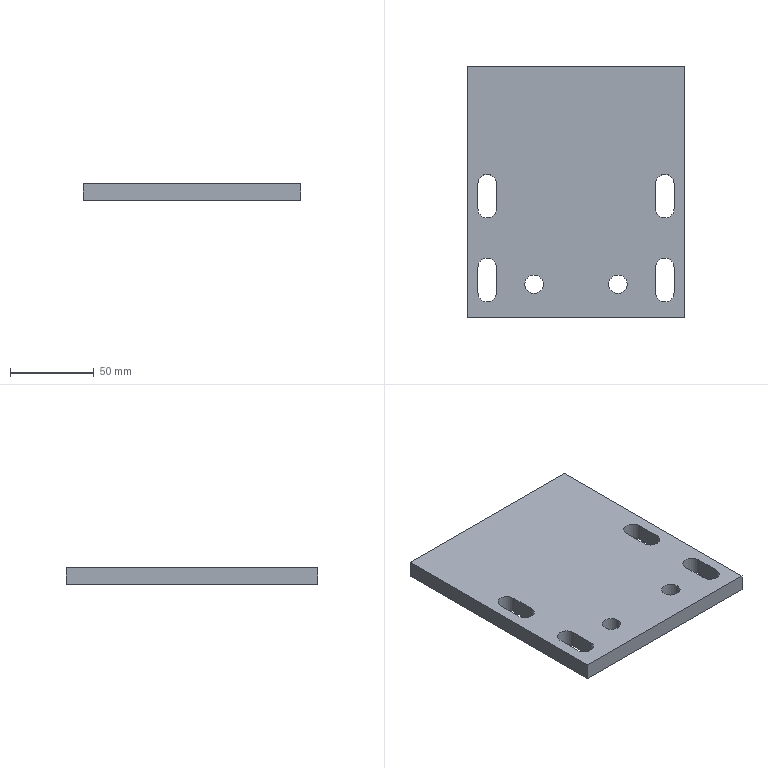Part | SolidWorks | features HoleWzd 2, ICE 2, Extrusion 1 | 1 solid | 26 faces | box 130 x 150 x 10 mm | volume 182698 mm3 | plane 14 | cylinder 12 | commonest cylinder face diameters 11 x12
STEP:
#1=CARTESIAN_POINT('',(34.5,20.,0.));
#2=VERTEX_POINT('',#1);
#3=CARTESIAN_POINT('',(45.5,20.,0.));
#4=VERTEX_POINT('',#3);
#5=CARTESIAN_POINT('',(40.,20.,0.));
#6=DIRECTION('',(0.,0.,1.));
#7=DIRECTION('',(1.,0.,0.));
#8=AXIS2_PLACEMENT_3D('',#5,#6,#7);
#9=CIRCLE('',#8,5.5);
#10=EDGE_CURVE('',#2,#4,#9,.T.);
#11=ORIENTED_EDGE('',*,*,#10,.F.);
#12=CARTESIAN_POINT('',(34.5,20.,10.));
#13=VERTEX_POINT('',#12);
#14=CARTESIAN_POINT('',(34.5,20.,10.));
#15=DIRECTION('',(0.,0.,1.));
#16=VECTOR('',#15,1000.);
#17=LINE('',#14,#16);
#18=EDGE_CURVE('',#2,#13,#17,.T.);
#19=ORIENTED_EDGE('',*,*,#18,.T.);
#20=CARTESIAN_POINT('',(45.5,20.,10.));
#21=VERTEX_POINT('',#20);
#22=CARTESIAN_POINT('',(40.,20.,10.));
#23=DIRECTION('',(0.,0.,1.));
#24=DIRECTION('',(1.,0.,0.));
#25=AXIS2_PLACEMENT_3D('',#22,#23,#24);
#26=CIRCLE('',#25,5.5);
#27=EDGE_CURVE('',#13,#21,#26,.T.);
#28=ORIENTED_EDGE('',*,*,#27,.T.);
#29=CARTESIAN_POINT('',(45.5,20.,10.));
#30=DIRECTION('',(0.,0.,1.));
#31=VECTOR('',#30,1000.);
#32=LINE('',#29,#31);
#33=EDGE_CURVE('',#4,#21,#32,.T.);
#34=ORIENTED_EDGE('',*,*,#33,.F.);
#35=EDGE_LOOP('',(#11,#19,#28,#34));
#36=FACE_OUTER_BOUND('',#35,.T.);
#37=CARTESIAN_POINT('',(40.,20.,10.));
#38=DIRECTION('',(0.,0.,1.));
#39=DIRECTION('',(1.,0.,0.));
#40=AXIS2_PLACEMENT_3D('',#37,#38,#39);
#41=CYLINDRICAL_SURFACE('',#40,5.5);
#42=ADVANCED_FACE('',(#36),#41,.F.);
#43=CARTESIAN_POINT('',(84.5,20.,0.));
#44=VERTEX_POINT('',#43);
#45=CARTESIAN_POINT('',(95.5,20.,0.));
#46=VERTEX_POINT('',#45);
#47=CARTESIAN_POINT('',(90.,20.,0.));
#48=DIRECTION('',(0.,0.,1.));
#49=DIRECTION('',(1.,0.,0.));
#50=AXIS2_PLACEMENT_3D('',#47,#48,#49);
#51=CIRCLE('',#50,5.5);
#52=EDGE_CURVE('',#44,#46,#51,.T.);
#53=ORIENTED_EDGE('',*,*,#52,.F.);
#54=CARTESIAN_POINT('',(84.5,20.,10.));
#55=VERTEX_POINT('',#54);
#56=CARTESIAN_POINT('',(84.5,20.,10.));
#57=DIRECTION('',(0.,0.,1.));
#58=VECTOR('',#57,1000.);
#59=LINE('',#56,#58);
#60=EDGE_CURVE('',#44,#55,#59,.T.);
#61=ORIENTED_EDGE('',*,*,#60,.T.);
#62=CARTESIAN_POINT('',(95.5,20.,10.));
#63=VERTEX_POINT('',#62);
#64=CARTESIAN_POINT('',(90.,20.,10.));
#65=DIRECTION('',(0.,0.,1.));
#66=DIRECTION('',(1.,0.,0.));
#67=AXIS2_PLACEMENT_3D('',#64,#65,#66);
#68=CIRCLE('',#67,5.5);
#69=EDGE_CURVE('',#55,#63,#68,.T.);
#70=ORIENTED_EDGE('',*,*,#69,.T.);
#71=CARTESIAN_POINT('',(95.5,20.,10.));
#72=DIRECTION('',(0.,0.,1.));
#73=VECTOR('',#72,1000.);
#74=LINE('',#71,#73);
#75=EDGE_CURVE('',#46,#63,#74,.T.);
#76=ORIENTED_EDGE('',*,*,#75,.F.);
#77=EDGE_LOOP('',(#53,#61,#70,#76));
#78=FACE_OUTER_BOUND('',#77,.T.);
#79=CARTESIAN_POINT('',(90.,20.,10.));
#80=DIRECTION('',(0.,0.,1.));
#81=DIRECTION('',(1.,0.,0.));
#82=AXIS2_PLACEMENT_3D('',#79,#80,#81);
#83=CYLINDRICAL_SURFACE('',#82,5.5);
#84=ADVANCED_FACE('',(#78),#83,.F.);
#85=CARTESIAN_POINT('',(0.,150.,0.));
#86=VERTEX_POINT('',#85);
#87=CARTESIAN_POINT('',(0.,0.,0.));
#88=VERTEX_POINT('',#87);
#89=CARTESIAN_POINT('',(0.,0.,0.));
#90=DIRECTION('',(0.,-1.,0.));
#91=VECTOR('',#90,1000.);
#92=LINE('',#89,#91);
#93=EDGE_CURVE('',#86,#88,#92,.T.);
#94=ORIENTED_EDGE('',*,*,#93,.T.);
#95=CARTESIAN_POINT('',(0.,0.,10.));
#96=VERTEX_POINT('',#95);
#97=CARTESIAN_POINT('',(0.,0.,10.));
#98=DIRECTION('',(0.,0.,-1.));
#99=VECTOR('',#98,1000.);
#100=LINE('',#97,#99);
#101=EDGE_CURVE('',#96,#88,#100,.T.);
#102=ORIENTED_EDGE('',*,*,#101,.F.);
#103=CARTESIAN_POINT('',(0.,150.,10.));
#104=VERTEX_POINT('',#103);
#105=CARTESIAN_POINT('',(0.,0.,10.));
#106=DIRECTION('',(0.,-1.,0.));
#107=VECTOR('',#106,1000.);
#108=LINE('',#105,#107);
#109=EDGE_CURVE('',#104,#96,#108,.T.);
#110=ORIENTED_EDGE('',*,*,#109,.F.);
#111=CARTESIAN_POINT('',(0.,150.,0.));
#112=DIRECTION('',(0.,0.,1.));
#113=VECTOR('',#112,1000.);
#114=LINE('',#111,#113);
#115=EDGE_CURVE('',#86,#104,#114,.T.);
#116=ORIENTED_EDGE('',*,*,#115,.F.);
#117=EDGE_LOOP('',(#94,#102,#110,#116));
#118=FACE_OUTER_BOUND('',#117,.T.);
#119=CARTESIAN_POINT('',(0.,0.,10.));
#120=DIRECTION('',(1.,0.,0.));
#121=DIRECTION('',(0.,0.,-1.));
#122=AXIS2_PLACEMENT_3D('',#119,#120,#121);
#123=PLANE('',#122);
#124=ADVANCED_FACE('',(#118),#123,.F.);
#125=CARTESIAN_POINT('',(130.,0.,0.));
#126=VERTEX_POINT('',#125);
#127=CARTESIAN_POINT('',(0.,0.,0.));
#128=DIRECTION('',(1.,0.,0.));
#129=VECTOR('',#128,1000.);
#130=LINE('',#127,#129);
#131=EDGE_CURVE('',#88,#126,#130,.T.);
#132=ORIENTED_EDGE('',*,*,#131,.T.);
#133=CARTESIAN_POINT('',(130.,0.,10.));
#134=VERTEX_POINT('',#133);
#135=CARTESIAN_POINT('',(130.,0.,10.));
#136=DIRECTION('',(0.,0.,-1.));
#137=VECTOR('',#136,1000.);
#138=LINE('',#135,#137);
#139=EDGE_CURVE('',#134,#126,#138,.T.);
#140=ORIENTED_EDGE('',*,*,#139,.F.);
#141=CARTESIAN_POINT('',(0.,0.,10.));
#142=DIRECTION('',(1.,0.,0.));
#143=VECTOR('',#142,1000.);
#144=LINE('',#141,#143);
#145=EDGE_CURVE('',#96,#134,#144,.T.);
#146=ORIENTED_EDGE('',*,*,#145,.F.);
#147=ORIENTED_EDGE('',*,*,#101,.T.);
#148=EDGE_LOOP('',(#132,#140,#146,#147));
#149=FACE_OUTER_BOUND('',#148,.T.);
#150=CARTESIAN_POINT('',(0.,0.,10.));
#151=DIRECTION('',(0.,1.,0.));
#152=DIRECTION('',(0.,0.,1.));
#153=AXIS2_PLACEMENT_3D('',#150,#151,#152);
#154=PLANE('',#153);
#155=ADVANCED_FACE('',(#149),#154,.F.);
#156=CARTESIAN_POINT('',(130.,150.,0.));
#157=VERTEX_POINT('',#156);
#158=CARTESIAN_POINT('',(130.,0.,0.));
#159=DIRECTION('',(0.,1.,0.));
#160=VECTOR('',#159,1000.);
#161=LINE('',#158,#160);
#162=EDGE_CURVE('',#126,#157,#161,.T.);
#163=ORIENTED_EDGE('',*,*,#162,.T.);
#164=CARTESIAN_POINT('',(130.,150.,10.));
#165=VERTEX_POINT('',#164);
#166=CARTESIAN_POINT('',(130.,150.,10.));
#167=DIRECTION('',(0.,0.,-1.));
#168=VECTOR('',#167,1000.);
#169=LINE('',#166,#168);
#170=EDGE_CURVE('',#165,#157,#169,.T.);
#171=ORIENTED_EDGE('',*,*,#170,.F.);
#172=CARTESIAN_POINT('',(130.,0.,10.));
#173=DIRECTION('',(0.,1.,0.));
#174=VECTOR('',#173,1000.);
#175=LINE('',#172,#174);
#176=EDGE_CURVE('',#134,#165,#175,.T.);
#177=ORIENTED_EDGE('',*,*,#176,.F.);
#178=ORIENTED_EDGE('',*,*,#139,.T.);
#179=EDGE_LOOP('',(#163,#171,#177,#178));
#180=FACE_OUTER_BOUND('',#179,.T.);
#181=CARTESIAN_POINT('',(130.,0.,10.));
#182=DIRECTION('',(-1.,0.,0.));
#183=DIRECTION('',(0.,0.,1.));
#184=AXIS2_PLACEMENT_3D('',#181,#182,#183);
#185=PLANE('',#184);
#186=ADVANCED_FACE('',(#180),#185,.F.);
#187=CARTESIAN_POINT('',(17.5,30.,10.));
#188=VERTEX_POINT('',#187);
#189=CARTESIAN_POINT('',(17.5,15.,10.));
#190=VERTEX_POINT('',#189);
#191=CARTESIAN_POINT('',(17.5,15.,10.));
#192=DIRECTION('',(0.,-1.,0.));
#193=VECTOR('',#192,1000.);
#194=LINE('',#191,#193);
#195=EDGE_CURVE('',#188,#190,#194,.T.);
#196=ORIENTED_EDGE('',*,*,#195,.T.);
#197=CARTESIAN_POINT('',(6.5,15.,10.));
#198=VERTEX_POINT('',#197);
#199=CARTESIAN_POINT('',(12.,15.,10.));
#200=DIRECTION('',(0.,0.,-1.));
#201=DIRECTION('',(-1.,0.,0.));
#202=AXIS2_PLACEMENT_3D('',#199,#200,#201);
#203=CIRCLE('',#202,5.5);
#204=EDGE_CURVE('',#190,#198,#203,.T.);
#205=ORIENTED_EDGE('',*,*,#204,.T.);
#206=CARTESIAN_POINT('',(6.5,30.,10.));
#207=VERTEX_POINT('',#206);
#208=CARTESIAN_POINT('',(6.5,15.,10.));
#209=DIRECTION('',(0.,1.,0.));
#210=VECTOR('',#209,1000.);
#211=LINE('',#208,#210);
#212=EDGE_CURVE('',#198,#207,#211,.T.);
#213=ORIENTED_EDGE('',*,*,#212,.T.);
#214=CARTESIAN_POINT('',(12.,30.,10.));
#215=DIRECTION('',(0.,0.,-1.));
#216=DIRECTION('',(-1.,0.,0.));
#217=AXIS2_PLACEMENT_3D('',#214,#215,#216);
#218=CIRCLE('',#217,5.5);
#219=EDGE_CURVE('',#207,#188,#218,.T.);
#220=ORIENTED_EDGE('',*,*,#219,.T.);
#221=EDGE_LOOP('',(#196,#205,#213,#220));
#222=FACE_BOUND('',#221,.T.);
#223=CARTESIAN_POINT('',(17.5,80.,10.));
#224=VERTEX_POINT('',#223);
#225=CARTESIAN_POINT('',(17.5,65.,10.));
#226=VERTEX_POINT('',#225);
#227=CARTESIAN_POINT('',(17.5,65.,10.));
#228=DIRECTION('',(0.,-1.,0.));
#229=VECTOR('',#228,1000.);
#230=LINE('',#227,#229);
#231=EDGE_CURVE('',#224,#226,#230,.T.);
#232=ORIENTED_EDGE('',*,*,#231,.T.);
#233=CARTESIAN_POINT('',(6.5,65.,10.));
#234=VERTEX_POINT('',#233);
#235=CARTESIAN_POINT('',(12.,65.,10.));
#236=DIRECTION('',(0.,0.,-1.));
#237=DIRECTION('',(-1.,0.,0.));
#238=AXIS2_PLACEMENT_3D('',#235,#236,#237);
#239=CIRCLE('',#238,5.5);
#240=EDGE_CURVE('',#226,#234,#239,.T.);
#241=ORIENTED_EDGE('',*,*,#240,.T.);
#242=CARTESIAN_POINT('',(6.5,80.,10.));
#243=VERTEX_POINT('',#242);
#244=CARTESIAN_POINT('',(6.5,65.,10.));
#245=DIRECTION('',(0.,1.,0.));
#246=VECTOR('',#245,1000.);
#247=LINE('',#244,#246);
#248=EDGE_CURVE('',#234,#243,#247,.T.);
#249=ORIENTED_EDGE('',*,*,#248,.T.);
#250=CARTESIAN_POINT('',(12.,80.,10.));
#251=DIRECTION('',(0.,0.,-1.));
#252=DIRECTION('',(-1.,0.,0.));
#253=AXIS2_PLACEMENT_3D('',#250,#251,#252);
#254=CIRCLE('',#253,5.5);
#255=EDGE_CURVE('',#243,#224,#254,.T.);
#256=ORIENTED_EDGE('',*,*,#255,.T.);
#257=EDGE_LOOP('',(#232,#241,#249,#256));
#258=FACE_BOUND('',#257,.T.);
#259=CARTESIAN_POINT('',(123.5,80.,10.));
#260=VERTEX_POINT('',#259);
#261=CARTESIAN_POINT('',(123.5,65.,10.));
#262=VERTEX_POINT('',#261);
#263=CARTESIAN_POINT('',(123.5,65.,10.));
#264=DIRECTION('',(0.,-1.,0.));
#265=VECTOR('',#264,1000.);
#266=LINE('',#263,#265);
#267=EDGE_CURVE('',#260,#262,#266,.T.);
#268=ORIENTED_EDGE('',*,*,#267,.T.);
#269=CARTESIAN_POINT('',(112.5,65.,10.));
#270=VERTEX_POINT('',#269);
#271=CARTESIAN_POINT('',(118.,65.,10.));
#272=DIRECTION('',(0.,0.,-1.));
#273=DIRECTION('',(-1.,0.,0.));
#274=AXIS2_PLACEMENT_3D('',#271,#272,#273);
#275=CIRCLE('',#274,5.5);
#276=EDGE_CURVE('',#262,#270,#275,.T.);
#277=ORIENTED_EDGE('',*,*,#276,.T.);
#278=CARTESIAN_POINT('',(112.5,80.,10.));
#279=VERTEX_POINT('',#278);
#280=CARTESIAN_POINT('',(112.5,65.,10.));
#281=DIRECTION('',(0.,1.,0.));
#282=VECTOR('',#281,1000.);
#283=LINE('',#280,#282);
#284=EDGE_CURVE('',#270,#279,#283,.T.);
#285=ORIENTED_EDGE('',*,*,#284,.T.);
#286=CARTESIAN_POINT('',(118.,80.,10.));
#287=DIRECTION('',(0.,0.,-1.));
#288=DIRECTION('',(-1.,0.,0.));
#289=AXIS2_PLACEMENT_3D('',#286,#287,#288);
#290=CIRCLE('',#289,5.5);
#291=EDGE_CURVE('',#279,#260,#290,.T.);
#292=ORIENTED_EDGE('',*,*,#291,.T.);
#293=EDGE_LOOP('',(#268,#277,#285,#292));
#294=FACE_BOUND('',#293,.T.);
#295=CARTESIAN_POINT('',(123.5,30.,10.));
#296=VERTEX_POINT('',#295);
#297=CARTESIAN_POINT('',(123.5,15.,10.));
#298=VERTEX_POINT('',#297);
#299=CARTESIAN_POINT('',(123.5,15.,10.));
#300=DIRECTION('',(0.,-1.,0.));
#301=VECTOR('',#300,1000.);
#302=LINE('',#299,#301);
#303=EDGE_CURVE('',#296,#298,#302,.T.);
#304=ORIENTED_EDGE('',*,*,#303,.T.);
#305=CARTESIAN_POINT('',(112.5,15.,10.));
#306=VERTEX_POINT('',#305);
#307=CARTESIAN_POINT('',(118.,15.,10.));
#308=DIRECTION('',(0.,0.,-1.));
#309=DIRECTION('',(-1.,0.,0.));
#310=AXIS2_PLACEMENT_3D('',#307,#308,#309);
#311=CIRCLE('',#310,5.5);
#312=EDGE_CURVE('',#298,#306,#311,.T.);
#313=ORIENTED_EDGE('',*,*,#312,.T.);
#314=CARTESIAN_POINT('',(112.5,30.,10.));
#315=VERTEX_POINT('',#314);
#316=CARTESIAN_POINT('',(112.5,15.,10.));
#317=DIRECTION('',(0.,1.,0.));
#318=VECTOR('',#317,1000.);
#319=LINE('',#316,#318);
#320=EDGE_CURVE('',#306,#315,#319,.T.);
#321=ORIENTED_EDGE('',*,*,#320,.T.);
#322=CARTESIAN_POINT('',(118.,30.,10.));
#323=DIRECTION('',(0.,0.,-1.));
#324=DIRECTION('',(-1.,0.,0.));
#325=AXIS2_PLACEMENT_3D('',#322,#323,#324);
#326=CIRCLE('',#325,5.5);
#327=EDGE_CURVE('',#315,#296,#326,.T.);
#328=ORIENTED_EDGE('',*,*,#327,.T.);
#329=EDGE_LOOP('',(#304,#313,#321,#328));
#330=FACE_BOUND('',#329,.T.);
#331=CARTESIAN_POINT('',(40.,20.,10.));
#332=DIRECTION('',(0.,0.,1.));
#333=DIRECTION('',(1.,0.,0.));
#334=AXIS2_PLACEMENT_3D('',#331,#332,#333);
#335=CIRCLE('',#334,5.5);
#336=EDGE_CURVE('',#21,#13,#335,.T.);
#337=ORIENTED_EDGE('',*,*,#336,.F.);
#338=ORIENTED_EDGE('',*,*,#27,.F.);
#339=EDGE_LOOP('',(#337,#338));
#340=FACE_BOUND('',#339,.T.);
#341=CARTESIAN_POINT('',(90.,20.,10.));
#342=DIRECTION('',(0.,0.,1.));
#343=DIRECTION('',(1.,0.,0.));
#344=AXIS2_PLACEMENT_3D('',#341,#342,#343);
#345=CIRCLE('',#344,5.5);
#346=EDGE_CURVE('',#63,#55,#345,.T.);
#347=ORIENTED_EDGE('',*,*,#346,.F.);
#348=ORIENTED_EDGE('',*,*,#69,.F.);
#349=EDGE_LOOP('',(#347,#348));
#350=FACE_BOUND('',#349,.T.);
#351=ORIENTED_EDGE('',*,*,#109,.T.);
#352=ORIENTED_EDGE('',*,*,#145,.T.);
#353=ORIENTED_EDGE('',*,*,#176,.T.);
#354=CARTESIAN_POINT('',(0.,150.,10.));
#355=DIRECTION('',(1.,0.,0.));
#356=VECTOR('',#355,1000.);
#357=LINE('',#354,#356);
#358=EDGE_CURVE('',#104,#165,#357,.T.);
#359=ORIENTED_EDGE('',*,*,#358,.F.);
#360=EDGE_LOOP('',(#351,#352,#353,#359));
#361=FACE_OUTER_BOUND('',#360,.T.);
#362=CARTESIAN_POINT('',(0.,0.,10.));
#363=DIRECTION('',(0.,0.,-1.));
#364=DIRECTION('',(-1.,0.,0.));
#365=AXIS2_PLACEMENT_3D('',#362,#363,#364);
#366=PLANE('',#365);
#367=ADVANCED_FACE('',(#222,#258,#294,#330,#340,#350,#361),#366,.F.);
#368=CARTESIAN_POINT('',(17.5,15.,0.));
#369=VERTEX_POINT('',#368);
#370=CARTESIAN_POINT('',(6.5,15.,0.));
#371=VERTEX_POINT('',#370);
#372=CARTESIAN_POINT('',(12.,15.,0.));
#373=DIRECTION('',(0.,0.,-1.));
#374=DIRECTION('',(-1.,0.,0.));
#375=AXIS2_PLACEMENT_3D('',#372,#373,#374);
#376=CIRCLE('',#375,5.5);
#377=EDGE_CURVE('',#369,#371,#376,.T.);
#378=ORIENTED_EDGE('',*,*,#377,.F.);
#379=CARTESIAN_POINT('',(17.5,30.,0.));
#380=VERTEX_POINT('',#379);
#381=CARTESIAN_POINT('',(17.5,15.,0.));
#382=DIRECTION('',(0.,-1.,0.));
#383=VECTOR('',#382,1000.);
#384=LINE('',#381,#383);
#385=EDGE_CURVE('',#380,#369,#384,.T.);
#386=ORIENTED_EDGE('',*,*,#385,.F.);
#387=CARTESIAN_POINT('',(6.5,30.,0.));
#388=VERTEX_POINT('',#387);
#389=CARTESIAN_POINT('',(12.,30.,0.));
#390=DIRECTION('',(0.,0.,-1.));
#391=DIRECTION('',(-1.,0.,0.));
#392=AXIS2_PLACEMENT_3D('',#389,#390,#391);
#393=CIRCLE('',#392,5.5);
#394=EDGE_CURVE('',#388,#380,#393,.T.);
#395=ORIENTED_EDGE('',*,*,#394,.F.);
#396=CARTESIAN_POINT('',(6.5,15.,0.));
#397=DIRECTION('',(0.,1.,0.));
#398=VECTOR('',#397,1000.);
#399=LINE('',#396,#398);
#400=EDGE_CURVE('',#371,#388,#399,.T.);
#401=ORIENTED_EDGE('',*,*,#400,.F.);
#402=EDGE_LOOP('',(#378,#386,#395,#401));
#403=FACE_BOUND('',#402,.T.);
#404=CARTESIAN_POINT('',(17.5,65.,0.));
#405=VERTEX_POINT('',#404);
#406=CARTESIAN_POINT('',(6.5,65.,0.));
#407=VERTEX_POINT('',#406);
#408=CARTESIAN_POINT('',(12.,65.,0.));
#409=DIRECTION('',(0.,0.,-1.));
#410=DIRECTION('',(-1.,0.,0.));
#411=AXIS2_PLACEMENT_3D('',#408,#409,#410);
#412=CIRCLE('',#411,5.5);
#413=EDGE_CURVE('',#405,#407,#412,.T.);
#414=ORIENTED_EDGE('',*,*,#413,.F.);
#415=CARTESIAN_POINT('',(17.5,80.,0.));
#416=VERTEX_POINT('',#415);
#417=CARTESIAN_POINT('',(17.5,65.,0.));
#418=DIRECTION('',(0.,-1.,0.));
#419=VECTOR('',#418,1000.);
#420=LINE('',#417,#419);
#421=EDGE_CURVE('',#416,#405,#420,.T.);
#422=ORIENTED_EDGE('',*,*,#421,.F.);
#423=CARTESIAN_POINT('',(6.5,80.,0.));
#424=VERTEX_POINT('',#423);
#425=CARTESIAN_POINT('',(12.,80.,0.));
#426=DIRECTION('',(0.,0.,-1.));
#427=DIRECTION('',(-1.,0.,0.));
#428=AXIS2_PLACEMENT_3D('',#425,#426,#427);
#429=CIRCLE('',#428,5.5);
#430=EDGE_CURVE('',#424,#416,#429,.T.);
#431=ORIENTED_EDGE('',*,*,#430,.F.);
#432=CARTESIAN_POINT('',(6.5,65.,0.));
#433=DIRECTION('',(0.,1.,0.));
#434=VECTOR('',#433,1000.);
#435=LINE('',#432,#434);
#436=EDGE_CURVE('',#407,#424,#435,.T.);
#437=ORIENTED_EDGE('',*,*,#436,.F.);
#438=EDGE_LOOP('',(#414,#422,#431,#437));
#439=FACE_BOUND('',#438,.T.);
#440=CARTESIAN_POINT('',(123.5,65.,0.));
#441=VERTEX_POINT('',#440);
#442=CARTESIAN_POINT('',(112.5,65.,0.));
#443=VERTEX_POINT('',#442);
#444=CARTESIAN_POINT('',(118.,65.,0.));
#445=DIRECTION('',(0.,0.,-1.));
#446=DIRECTION('',(-1.,0.,0.));
#447=AXIS2_PLACEMENT_3D('',#444,#445,#446);
#448=CIRCLE('',#447,5.5);
#449=EDGE_CURVE('',#441,#443,#448,.T.);
#450=ORIENTED_EDGE('',*,*,#449,.F.);
#451=CARTESIAN_POINT('',(123.5,80.,0.));
#452=VERTEX_POINT('',#451);
#453=CARTESIAN_POINT('',(123.5,65.,0.));
#454=DIRECTION('',(0.,-1.,0.));
#455=VECTOR('',#454,1000.);
#456=LINE('',#453,#455);
#457=EDGE_CURVE('',#452,#441,#456,.T.);
#458=ORIENTED_EDGE('',*,*,#457,.F.);
#459=CARTESIAN_POINT('',(112.5,80.,0.));
#460=VERTEX_POINT('',#459);
#461=CARTESIAN_POINT('',(118.,80.,0.));
#462=DIRECTION('',(0.,0.,-1.));
#463=DIRECTION('',(-1.,0.,0.));
#464=AXIS2_PLACEMENT_3D('',#461,#462,#463);
#465=CIRCLE('',#464,5.5);
#466=EDGE_CURVE('',#460,#452,#465,.T.);
#467=ORIENTED_EDGE('',*,*,#466,.F.);
#468=CARTESIAN_POINT('',(112.5,65.,0.));
#469=DIRECTION('',(0.,1.,0.));
#470=VECTOR('',#469,1000.);
#471=LINE('',#468,#470);
#472=EDGE_CURVE('',#443,#460,#471,.T.);
#473=ORIENTED_EDGE('',*,*,#472,.F.);
#474=EDGE_LOOP('',(#450,#458,#467,#473));
#475=FACE_BOUND('',#474,.T.);
#476=CARTESIAN_POINT('',(123.5,15.,0.));
#477=VERTEX_POINT('',#476);
#478=CARTESIAN_POINT('',(112.5,15.,0.));
#479=VERTEX_POINT('',#478);
#480=CARTESIAN_POINT('',(118.,15.,0.));
#481=DIRECTION('',(0.,0.,-1.));
#482=DIRECTION('',(-1.,0.,0.));
#483=AXIS2_PLACEMENT_3D('',#480,#481,#482);
#484=CIRCLE('',#483,5.5);
#485=EDGE_CURVE('',#477,#479,#484,.T.);
#486=ORIENTED_EDGE('',*,*,#485,.F.);
#487=CARTESIAN_POINT('',(123.5,30.,0.));
#488=VERTEX_POINT('',#487);
#489=CARTESIAN_POINT('',(123.5,15.,0.));
#490=DIRECTION('',(0.,-1.,0.));
#491=VECTOR('',#490,1000.);
#492=LINE('',#489,#491);
#493=EDGE_CURVE('',#488,#477,#492,.T.);
#494=ORIENTED_EDGE('',*,*,#493,.F.);
#495=CARTESIAN_POINT('',(112.5,30.,0.));
#496=VERTEX_POINT('',#495);
#497=CARTESIAN_POINT('',(118.,30.,0.));
#498=DIRECTION('',(0.,0.,-1.));
#499=DIRECTION('',(-1.,0.,0.));
#500=AXIS2_PLACEMENT_3D('',#497,#498,#499);
#501=CIRCLE('',#500,5.5);
#502=EDGE_CURVE('',#496,#488,#501,.T.);
#503=ORIENTED_EDGE('',*,*,#502,.F.);
#504=CARTESIAN_POINT('',(112.5,15.,0.));
#505=DIRECTION('',(0.,1.,0.));
#506=VECTOR('',#505,1000.);
#507=LINE('',#504,#506);
#508=EDGE_CURVE('',#479,#496,#507,.T.);
#509=ORIENTED_EDGE('',*,*,#508,.F.);
#510=EDGE_LOOP('',(#486,#494,#503,#509));
#511=FACE_BOUND('',#510,.T.);
#512=CARTESIAN_POINT('',(40.,20.,0.));
#513=DIRECTION('',(0.,0.,1.));
#514=DIRECTION('',(1.,0.,0.));
#515=AXIS2_PLACEMENT_3D('',#512,#513,#514);
#516=CIRCLE('',#515,5.5);
#517=EDGE_CURVE('',#4,#2,#516,.T.);
#518=ORIENTED_EDGE('',*,*,#517,.T.);
#519=ORIENTED_EDGE('',*,*,#10,.T.);
#520=EDGE_LOOP('',(#518,#519));
#521=FACE_BOUND('',#520,.T.);
#522=CARTESIAN_POINT('',(90.,20.,0.));
#523=DIRECTION('',(0.,0.,1.));
#524=DIRECTION('',(1.,0.,0.));
#525=AXIS2_PLACEMENT_3D('',#522,#523,#524);
#526=CIRCLE('',#525,5.5);
#527=EDGE_CURVE('',#46,#44,#526,.T.);
#528=ORIENTED_EDGE('',*,*,#527,.T.);
#529=ORIENTED_EDGE('',*,*,#52,.T.);
#530=EDGE_LOOP('',(#528,#529));
#531=FACE_BOUND('',#530,.T.);
#532=ORIENTED_EDGE('',*,*,#93,.F.);
#533=CARTESIAN_POINT('',(130.,150.,0.));
#534=DIRECTION('',(-1.,0.,0.));
#535=VECTOR('',#534,1000.);
#536=LINE('',#533,#535);
#537=EDGE_CURVE('',#157,#86,#536,.T.);
#538=ORIENTED_EDGE('',*,*,#537,.F.);
#539=ORIENTED_EDGE('',*,*,#162,.F.);
#540=ORIENTED_EDGE('',*,*,#131,.F.);
#541=EDGE_LOOP('',(#532,#538,#539,#540));
#542=FACE_OUTER_BOUND('',#541,.T.);
#543=CARTESIAN_POINT('',(0.,0.,0.));
#544=DIRECTION('',(0.,0.,-1.));
#545=DIRECTION('',(-1.,0.,0.));
#546=AXIS2_PLACEMENT_3D('',#543,#544,#545);
#547=PLANE('',#546);
#548=ADVANCED_FACE('',(#403,#439,#475,#511,#521,#531,#542),#547,.T.);
#549=ORIENTED_EDGE('',*,*,#60,.F.);
#550=ORIENTED_EDGE('',*,*,#527,.F.);
#551=ORIENTED_EDGE('',*,*,#75,.T.);
#552=ORIENTED_EDGE('',*,*,#346,.T.);
#553=EDGE_LOOP('',(#549,#550,#551,#552));
#554=FACE_OUTER_BOUND('',#553,.T.);
#555=CARTESIAN_POINT('',(90.,20.,10.));
#556=DIRECTION('',(0.,0.,1.));
#557=DIRECTION('',(1.,0.,0.));
#558=AXIS2_PLACEMENT_3D('',#555,#556,#557);
#559=CYLINDRICAL_SURFACE('',#558,5.5);
#560=ADVANCED_FACE('',(#554),#559,.F.);
#561=ORIENTED_EDGE('',*,*,#18,.F.);
#562=ORIENTED_EDGE('',*,*,#517,.F.);
#563=ORIENTED_EDGE('',*,*,#33,.T.);
#564=ORIENTED_EDGE('',*,*,#336,.T.);
#565=EDGE_LOOP('',(#561,#562,#563,#564));
#566=FACE_OUTER_BOUND('',#565,.T.);
#567=CARTESIAN_POINT('',(40.,20.,10.));
#568=DIRECTION('',(0.,0.,1.));
#569=DIRECTION('',(1.,0.,0.));
#570=AXIS2_PLACEMENT_3D('',#567,#568,#569);
#571=CYLINDRICAL_SURFACE('',#570,5.5);
#572=ADVANCED_FACE('',(#566),#571,.F.);
#573=ORIENTED_EDGE('',*,*,#170,.T.);
#574=ORIENTED_EDGE('',*,*,#537,.T.);
#575=ORIENTED_EDGE('',*,*,#115,.T.);
#576=ORIENTED_EDGE('',*,*,#358,.T.);
#577=EDGE_LOOP('',(#573,#574,#575,#576));
#578=FACE_OUTER_BOUND('',#577,.T.);
#579=CARTESIAN_POINT('',(0.,150.,0.));
#580=DIRECTION('',(0.,1.,0.));
#581=DIRECTION('',(0.,0.,1.));
#582=AXIS2_PLACEMENT_3D('',#579,#580,#581);
#583=PLANE('',#582);
#584=ADVANCED_FACE('',(#578),#583,.T.);
#585=ORIENTED_EDGE('',*,*,#485,.T.);
#586=CARTESIAN_POINT('',(112.5,15.,10.));
#587=DIRECTION('',(0.,0.,-1.));
#588=VECTOR('',#587,1000.);
#589=LINE('',#586,#588);
#590=EDGE_CURVE('',#306,#479,#589,.T.);
#591=ORIENTED_EDGE('',*,*,#590,.F.);
#592=ORIENTED_EDGE('',*,*,#312,.F.);
#593=CARTESIAN_POINT('',(123.5,15.,10.));
#594=DIRECTION('',(0.,0.,-1.));
#595=VECTOR('',#594,1000.);
#596=LINE('',#593,#595);
#597=EDGE_CURVE('',#298,#477,#596,.T.);
#598=ORIENTED_EDGE('',*,*,#597,.T.);
#599=EDGE_LOOP('',(#585,#591,#592,#598));
#600=FACE_OUTER_BOUND('',#599,.T.);
#601=CARTESIAN_POINT('',(118.,15.,10.));
#602=DIRECTION('',(0.,0.,-1.));
#603=DIRECTION('',(-1.,0.,0.));
#604=AXIS2_PLACEMENT_3D('',#601,#602,#603);
#605=CYLINDRICAL_SURFACE('',#604,5.5);
#606=ADVANCED_FACE('',(#600),#605,.F.);
#607=ORIENTED_EDGE('',*,*,#493,.T.);
#608=ORIENTED_EDGE('',*,*,#597,.F.);
#609=ORIENTED_EDGE('',*,*,#303,.F.);
#610=CARTESIAN_POINT('',(123.5,30.,10.));
#611=DIRECTION('',(0.,0.,-1.));
#612=VECTOR('',#611,1000.);
#613=LINE('',#610,#612);
#614=EDGE_CURVE('',#296,#488,#613,.T.);
#615=ORIENTED_EDGE('',*,*,#614,.T.);
#616=EDGE_LOOP('',(#607,#608,#609,#615));
#617=FACE_OUTER_BOUND('',#616,.T.);
#618=CARTESIAN_POINT('',(123.5,15.,10.));
#619=DIRECTION('',(1.,0.,0.));
#620=DIRECTION('',(0.,0.,-1.));
#621=AXIS2_PLACEMENT_3D('',#618,#619,#620);
#622=PLANE('',#621);
#623=ADVANCED_FACE('',(#617),#622,.F.);
#624=ORIENTED_EDGE('',*,*,#502,.T.);
#625=ORIENTED_EDGE('',*,*,#614,.F.);
#626=ORIENTED_EDGE('',*,*,#327,.F.);
#627=CARTESIAN_POINT('',(112.5,30.,10.));
#628=DIRECTION('',(0.,0.,-1.));
#629=VECTOR('',#628,1000.);
#630=LINE('',#627,#629);
#631=EDGE_CURVE('',#315,#496,#630,.T.);
#632=ORIENTED_EDGE('',*,*,#631,.T.);
#633=EDGE_LOOP('',(#624,#625,#626,#632));
#634=FACE_OUTER_BOUND('',#633,.T.);
#635=CARTESIAN_POINT('',(118.,30.,10.));
#636=DIRECTION('',(0.,0.,-1.));
#637=DIRECTION('',(-1.,0.,0.));
#638=AXIS2_PLACEMENT_3D('',#635,#636,#637);
#639=CYLINDRICAL_SURFACE('',#638,5.5);
#640=ADVANCED_FACE('',(#634),#639,.F.);
#641=ORIENTED_EDGE('',*,*,#508,.T.);
#642=ORIENTED_EDGE('',*,*,#631,.F.);
#643=ORIENTED_EDGE('',*,*,#320,.F.);
#644=ORIENTED_EDGE('',*,*,#590,.T.);
#645=EDGE_LOOP('',(#641,#642,#643,#644));
#646=FACE_OUTER_BOUND('',#645,.T.);
#647=CARTESIAN_POINT('',(112.5,15.,10.));
#648=DIRECTION('',(-1.,0.,0.));
#649=DIRECTION('',(0.,0.,1.));
#650=AXIS2_PLACEMENT_3D('',#647,#648,#649);
#651=PLANE('',#650);
#652=ADVANCED_FACE('',(#646),#651,.F.);
#653=ORIENTED_EDGE('',*,*,#449,.T.);
#654=CARTESIAN_POINT('',(112.5,65.,10.));
#655=DIRECTION('',(0.,0.,-1.));
#656=VECTOR('',#655,1000.);
#657=LINE('',#654,#656);
#658=EDGE_CURVE('',#270,#443,#657,.T.);
#659=ORIENTED_EDGE('',*,*,#658,.F.);
#660=ORIENTED_EDGE('',*,*,#276,.F.);
#661=CARTESIAN_POINT('',(123.5,65.,10.));
#662=DIRECTION('',(0.,0.,-1.));
#663=VECTOR('',#662,1000.);
#664=LINE('',#661,#663);
#665=EDGE_CURVE('',#262,#441,#664,.T.);
#666=ORIENTED_EDGE('',*,*,#665,.T.);
#667=EDGE_LOOP('',(#653,#659,#660,#666));
#668=FACE_OUTER_BOUND('',#667,.T.);
#669=CARTESIAN_POINT('',(118.,65.,10.));
#670=DIRECTION('',(0.,0.,-1.));
#671=DIRECTION('',(-1.,0.,0.));
#672=AXIS2_PLACEMENT_3D('',#669,#670,#671);
#673=CYLINDRICAL_SURFACE('',#672,5.5);
#674=ADVANCED_FACE('',(#668),#673,.F.);
#675=ORIENTED_EDGE('',*,*,#457,.T.);
#676=ORIENTED_EDGE('',*,*,#665,.F.);
#677=ORIENTED_EDGE('',*,*,#267,.F.);
#678=CARTESIAN_POINT('',(123.5,80.,10.));
#679=DIRECTION('',(0.,0.,-1.));
#680=VECTOR('',#679,1000.);
#681=LINE('',#678,#680);
#682=EDGE_CURVE('',#260,#452,#681,.T.);
#683=ORIENTED_EDGE('',*,*,#682,.T.);
#684=EDGE_LOOP('',(#675,#676,#677,#683));
#685=FACE_OUTER_BOUND('',#684,.T.);
#686=CARTESIAN_POINT('',(123.5,65.,10.));
#687=DIRECTION('',(1.,0.,0.));
#688=DIRECTION('',(0.,0.,-1.));
#689=AXIS2_PLACEMENT_3D('',#686,#687,#688);
#690=PLANE('',#689);
#691=ADVANCED_FACE('',(#685),#690,.F.);
#692=ORIENTED_EDGE('',*,*,#466,.T.);
#693=ORIENTED_EDGE('',*,*,#682,.F.);
#694=ORIENTED_EDGE('',*,*,#291,.F.);
#695=CARTESIAN_POINT('',(112.5,80.,10.));
#696=DIRECTION('',(0.,0.,-1.));
#697=VECTOR('',#696,1000.);
#698=LINE('',#695,#697);
#699=EDGE_CURVE('',#279,#460,#698,.T.);
#700=ORIENTED_EDGE('',*,*,#699,.T.);
#701=EDGE_LOOP('',(#692,#693,#694,#700));
#702=FACE_OUTER_BOUND('',#701,.T.);
#703=CARTESIAN_POINT('',(118.,80.,10.));
#704=DIRECTION('',(0.,0.,-1.));
#705=DIRECTION('',(-1.,0.,0.));
#706=AXIS2_PLACEMENT_3D('',#703,#704,#705);
#707=CYLINDRICAL_SURFACE('',#706,5.5);
#708=ADVANCED_FACE('',(#702),#707,.F.);
#709=ORIENTED_EDGE('',*,*,#472,.T.);
#710=ORIENTED_EDGE('',*,*,#699,.F.);
#711=ORIENTED_EDGE('',*,*,#284,.F.);
#712=ORIENTED_EDGE('',*,*,#658,.T.);
#713=EDGE_LOOP('',(#709,#710,#711,#712));
#714=FACE_OUTER_BOUND('',#713,.T.);
#715=CARTESIAN_POINT('',(112.5,65.,10.));
#716=DIRECTION('',(-1.,0.,0.));
#717=DIRECTION('',(0.,0.,1.));
#718=AXIS2_PLACEMENT_3D('',#715,#716,#717);
#719=PLANE('',#718);
#720=ADVANCED_FACE('',(#714),#719,.F.);
#721=ORIENTED_EDGE('',*,*,#413,.T.);
#722=CARTESIAN_POINT('',(6.5,65.,10.));
#723=DIRECTION('',(0.,0.,-1.));
#724=VECTOR('',#723,1000.);
#725=LINE('',#722,#724);
#726=EDGE_CURVE('',#234,#407,#725,.T.);
#727=ORIENTED_EDGE('',*,*,#726,.F.);
#728=ORIENTED_EDGE('',*,*,#240,.F.);
#729=CARTESIAN_POINT('',(17.5,65.,10.));
#730=DIRECTION('',(0.,0.,-1.));
#731=VECTOR('',#730,1000.);
#732=LINE('',#729,#731);
#733=EDGE_CURVE('',#226,#405,#732,.T.);
#734=ORIENTED_EDGE('',*,*,#733,.T.);
#735=EDGE_LOOP('',(#721,#727,#728,#734));
#736=FACE_OUTER_BOUND('',#735,.T.);
#737=CARTESIAN_POINT('',(12.,65.,10.));
#738=DIRECTION('',(0.,0.,-1.));
#739=DIRECTION('',(-1.,0.,0.));
#740=AXIS2_PLACEMENT_3D('',#737,#738,#739);
#741=CYLINDRICAL_SURFACE('',#740,5.5);
#742=ADVANCED_FACE('',(#736),#741,.F.);
#743=ORIENTED_EDGE('',*,*,#421,.T.);
#744=ORIENTED_EDGE('',*,*,#733,.F.);
#745=ORIENTED_EDGE('',*,*,#231,.F.);
#746=CARTESIAN_POINT('',(17.5,80.,10.));
#747=DIRECTION('',(0.,0.,-1.));
#748=VECTOR('',#747,1000.);
#749=LINE('',#746,#748);
#750=EDGE_CURVE('',#224,#416,#749,.T.);
#751=ORIENTED_EDGE('',*,*,#750,.T.);
#752=EDGE_LOOP('',(#743,#744,#745,#751));
#753=FACE_OUTER_BOUND('',#752,.T.);
#754=CARTESIAN_POINT('',(17.5,65.,10.));
#755=DIRECTION('',(1.,0.,0.));
#756=DIRECTION('',(0.,1.,0.));
#757=AXIS2_PLACEMENT_3D('',#754,#755,#756);
#758=PLANE('',#757);
#759=ADVANCED_FACE('',(#753),#758,.F.);
#760=ORIENTED_EDGE('',*,*,#430,.T.);
#761=ORIENTED_EDGE('',*,*,#750,.F.);
#762=ORIENTED_EDGE('',*,*,#255,.F.);
#763=CARTESIAN_POINT('',(6.5,80.,10.));
#764=DIRECTION('',(0.,0.,-1.));
#765=VECTOR('',#764,1000.);
#766=LINE('',#763,#765);
#767=EDGE_CURVE('',#243,#424,#766,.T.);
#768=ORIENTED_EDGE('',*,*,#767,.T.);
#769=EDGE_LOOP('',(#760,#761,#762,#768));
#770=FACE_OUTER_BOUND('',#769,.T.);
#771=CARTESIAN_POINT('',(12.,80.,10.));
#772=DIRECTION('',(0.,0.,-1.));
#773=DIRECTION('',(-1.,0.,0.));
#774=AXIS2_PLACEMENT_3D('',#771,#772,#773);
#775=CYLINDRICAL_SURFACE('',#774,5.5);
#776=ADVANCED_FACE('',(#770),#775,.F.);
#777=ORIENTED_EDGE('',*,*,#436,.T.);
#778=ORIENTED_EDGE('',*,*,#767,.F.);
#779=ORIENTED_EDGE('',*,*,#248,.F.);
#780=ORIENTED_EDGE('',*,*,#726,.T.);
#781=EDGE_LOOP('',(#777,#778,#779,#780));
#782=FACE_OUTER_BOUND('',#781,.T.);
#783=CARTESIAN_POINT('',(6.5,65.,10.));
#784=DIRECTION('',(-1.,0.,0.));
#785=DIRECTION('',(0.,-1.,0.));
#786=AXIS2_PLACEMENT_3D('',#783,#784,#785);
#787=PLANE('',#786);
#788=ADVANCED_FACE('',(#782),#787,.F.);
#789=ORIENTED_EDGE('',*,*,#377,.T.);
#790=CARTESIAN_POINT('',(6.5,15.,10.));
#791=DIRECTION('',(0.,0.,-1.));
#792=VECTOR('',#791,1000.);
#793=LINE('',#790,#792);
#794=EDGE_CURVE('',#198,#371,#793,.T.);
#795=ORIENTED_EDGE('',*,*,#794,.F.);
#796=ORIENTED_EDGE('',*,*,#204,.F.);
#797=CARTESIAN_POINT('',(17.5,15.,10.));
#798=DIRECTION('',(0.,0.,-1.));
#799=VECTOR('',#798,1000.);
#800=LINE('',#797,#799);
#801=EDGE_CURVE('',#190,#369,#800,.T.);
#802=ORIENTED_EDGE('',*,*,#801,.T.);
#803=EDGE_LOOP('',(#789,#795,#796,#802));
#804=FACE_OUTER_BOUND('',#803,.T.);
#805=CARTESIAN_POINT('',(12.,15.,10.));
#806=DIRECTION('',(0.,0.,-1.));
#807=DIRECTION('',(-1.,0.,0.));
#808=AXIS2_PLACEMENT_3D('',#805,#806,#807);
#809=CYLINDRICAL_SURFACE('',#808,5.5);
#810=ADVANCED_FACE('',(#804),#809,.F.);
#811=ORIENTED_EDGE('',*,*,#385,.T.);
#812=ORIENTED_EDGE('',*,*,#801,.F.);
#813=ORIENTED_EDGE('',*,*,#195,.F.);
#814=CARTESIAN_POINT('',(17.5,30.,10.));
#815=DIRECTION('',(0.,0.,-1.));
#816=VECTOR('',#815,1000.);
#817=LINE('',#814,#816);
#818=EDGE_CURVE('',#188,#380,#817,.T.);
#819=ORIENTED_EDGE('',*,*,#818,.T.);
#820=EDGE_LOOP('',(#811,#812,#813,#819));
#821=FACE_OUTER_BOUND('',#820,.T.);
#822=CARTESIAN_POINT('',(17.5,15.,10.));
#823=DIRECTION('',(1.,0.,0.));
#824=DIRECTION('',(0.,1.,0.));
#825=AXIS2_PLACEMENT_3D('',#822,#823,#824);
#826=PLANE('',#825);
#827=ADVANCED_FACE('',(#821),#826,.F.);
#828=ORIENTED_EDGE('',*,*,#394,.T.);
#829=ORIENTED_EDGE('',*,*,#818,.F.);
#830=ORIENTED_EDGE('',*,*,#219,.F.);
#831=CARTESIAN_POINT('',(6.5,30.,10.));
#832=DIRECTION('',(0.,0.,-1.));
#833=VECTOR('',#832,1000.);
#834=LINE('',#831,#833);
#835=EDGE_CURVE('',#207,#388,#834,.T.);
#836=ORIENTED_EDGE('',*,*,#835,.T.);
#837=EDGE_LOOP('',(#828,#829,#830,#836));
#838=FACE_OUTER_BOUND('',#837,.T.);
#839=CARTESIAN_POINT('',(12.,30.,10.));
#840=DIRECTION('',(0.,0.,-1.));
#841=DIRECTION('',(-1.,0.,0.));
#842=AXIS2_PLACEMENT_3D('',#839,#840,#841);
#843=CYLINDRICAL_SURFACE('',#842,5.5);
#844=ADVANCED_FACE('',(#838),#843,.F.);
#845=ORIENTED_EDGE('',*,*,#400,.T.);
#846=ORIENTED_EDGE('',*,*,#835,.F.);
#847=ORIENTED_EDGE('',*,*,#212,.F.);
#848=ORIENTED_EDGE('',*,*,#794,.T.);
#849=EDGE_LOOP('',(#845,#846,#847,#848));
#850=FACE_OUTER_BOUND('',#849,.T.);
#851=CARTESIAN_POINT('',(6.5,15.,10.));
#852=DIRECTION('',(-1.,0.,0.));
#853=DIRECTION('',(0.,-1.,0.));
#854=AXIS2_PLACEMENT_3D('',#851,#852,#853);
#855=PLANE('',#854);
#856=ADVANCED_FACE('',(#850),#855,.F.);
#857=CLOSED_SHELL('',(#42,#84,#124,#155,#186,#367,#548,#560,#572,#584,#606,#623,#640,#652,#674,#691,#708,#720,#742,#759,#776,#788,#810,#827,#844,#856));
#858=MANIFOLD_SOLID_BREP('',#857);
#859=CARTESIAN_POINT('',(0.,0.,0.));
#860=DIRECTION('',(0.,0.,1.));
#861=DIRECTION('',(1.,0.,0.));
#862=AXIS2_PLACEMENT_3D('',#859,#860,#861);
#863=(LENGTH_UNIT()NAMED_UNIT(*)SI_UNIT(.MILLI.,.METRE.));
#864=UNCERTAINTY_MEASURE_WITH_UNIT(LENGTH_MEASURE(0.00001),#863,'','');
#865=(NAMED_UNIT(*)PLANE_ANGLE_UNIT()SI_UNIT($,.RADIAN.));
#866=(NAMED_UNIT(*)SI_UNIT($,.STERADIAN.)SOLID_ANGLE_UNIT());
#867=(GEOMETRIC_REPRESENTATION_CONTEXT(3)GLOBAL_UNCERTAINTY_ASSIGNED_CONTEXT((#864))GLOBAL_UNIT_ASSIGNED_CONTEXT((#863,#865,#866))REPRESENTATION_CONTEXT('',''));
#868=ADVANCED_BREP_SHAPE_REPRESENTATION('',(#858,#862),#867);